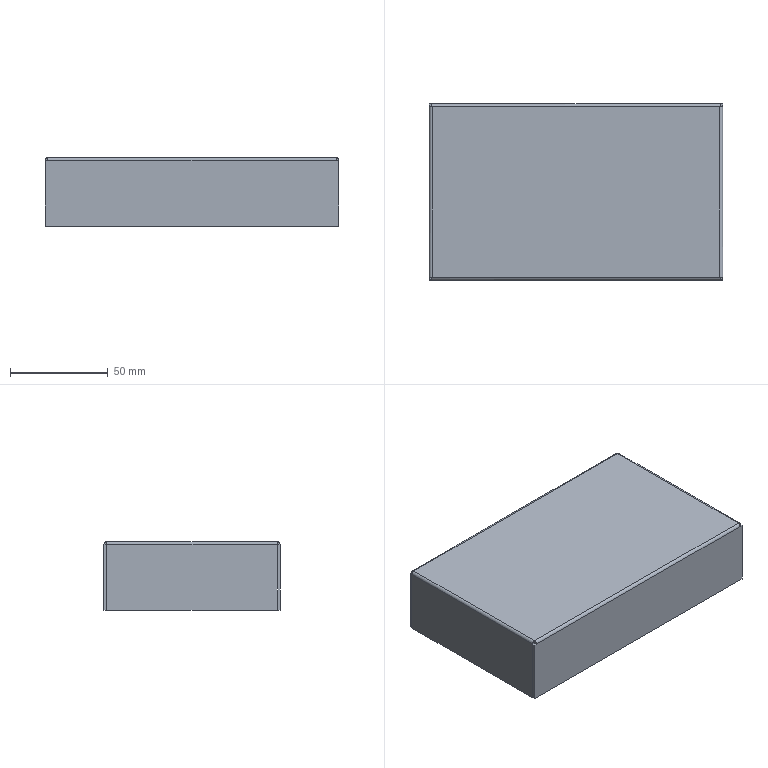Part | STEP file | FHD-021-007-D TZD10S drawer 4 | 1 solid | 48 faces | box 150 x 90 x 35 mm | volume 35026 mm3 | plane 30 | cylinder 10 | spline 8 | commonest cylinder face diameters 0.4 x4 2.8 x4 11 x2